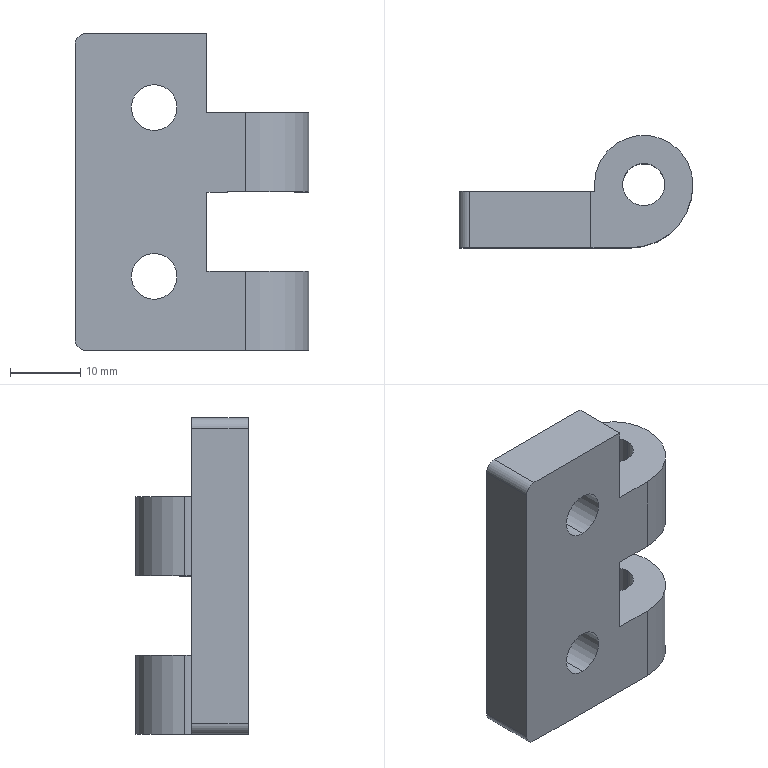Part | STEP file | _HFC01-45-002 | 1 solid | 30 faces | box 33.25 x 16 x 45 mm | volume 9553 mm3 | cylinder 16 | plane 10 | cone 4 | commonest cylinder face diameters 6 x4 6.5 x4 14 x4 3 x2 18 x2